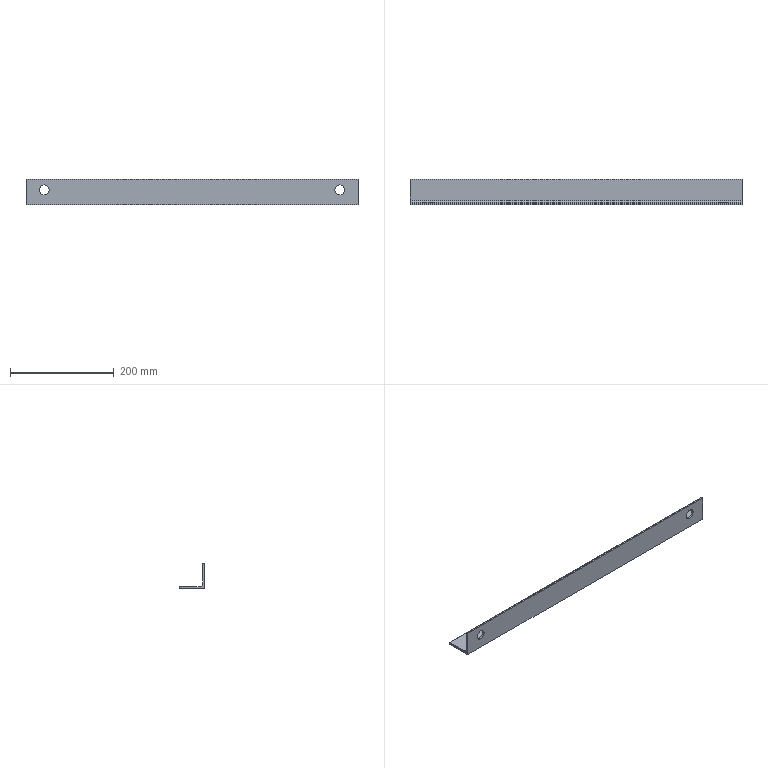Part | STEP file | 粉仓楼梯通道角钢_Default<As Machined> | 1 solid | 15 faces | box 640 x 50 x 50 mm | volume 247161 mm3 | plane 8 | cylinder 7 | commonest cylinder face diameters 19 x4 2.66 x2 11 x1
STEP:
#1=CARTESIAN_POINT('',(0.,0.,0.));
#2=DIRECTION('',(0.,0.,1.));
#3=DIRECTION('',(1.,0.,0.));
#4=AXIS2_PLACEMENT_3D('',#1,#2,#3);
#5=CARTESIAN_POINT('',(-285.,0.,38.585));
#6=VERTEX_POINT('',#5);
#7=CARTESIAN_POINT('',(-285.,4.,38.585));
#8=VERTEX_POINT('',#7);
#9=CARTESIAN_POINT('',(-285.,-6.,38.585));
#10=DIRECTION('',(0.,1.,0.));
#11=VECTOR('',#10,1.);
#12=LINE('',#9,#11);
#13=CARTESIAN_POINT('',(-285.,-6.,29.085));
#14=DIRECTION('',(0.,1.,0.));
#15=DIRECTION('',(0.,0.,1.));
#16=AXIS2_PLACEMENT_3D('',#13,#14,#15);
#17=CYLINDRICAL_SURFACE('',#16,9.5);
#18=CARTESIAN_POINT('',(6.283,0.));
#19=DIRECTION('',(0.,1.));
#20=VECTOR('',#19,1.);
#21=LINE('',#18,#20);
#22=(GEOMETRIC_REPRESENTATION_CONTEXT(2)PARAMETRIC_REPRESENTATION_CONTEXT()REPRESENTATION_CONTEXT('',''));
#23=DEFINITIONAL_REPRESENTATION('',(#21),#22);
#24=PCURVE('',#17,#23);
#25=CARTESIAN_POINT('',(-285.,-6.,29.085));
#26=DIRECTION('',(0.,1.,0.));
#27=DIRECTION('',(0.,0.,1.));
#28=AXIS2_PLACEMENT_3D('',#25,#26,#27);
#29=CYLINDRICAL_SURFACE('',#28,9.5);
#30=CARTESIAN_POINT('',(0.,0.));
#31=DIRECTION('',(0.,1.));
#32=VECTOR('',#31,1.);
#33=LINE('',#30,#32);
#34=(GEOMETRIC_REPRESENTATION_CONTEXT(2)PARAMETRIC_REPRESENTATION_CONTEXT()REPRESENTATION_CONTEXT('',''));
#35=DEFINITIONAL_REPRESENTATION('',(#33),#34);
#36=PCURVE('',#29,#35);
#37=SURFACE_CURVE('',#12,(#24,#36),.PCURVE_S1.);
#38=EDGE_CURVE('',#6,#8,#37,.T.);
#39=ORIENTED_EDGE('',*,*,#38,.T.);
#40=CARTESIAN_POINT('',(-285.,4.,19.585));
#41=VERTEX_POINT('',#40);
#42=CARTESIAN_POINT('',(-285.,4.,29.085));
#43=DIRECTION('',(0.,1.,0.));
#44=DIRECTION('',(0.,0.,1.));
#45=AXIS2_PLACEMENT_3D('',#42,#43,#44);
#46=CIRCLE('',#45,9.5);
#47=CARTESIAN_POINT('',(0.,10.));
#48=DIRECTION('',(1.,0.));
#49=VECTOR('',#48,1.);
#50=LINE('',#47,#49);
#51=(GEOMETRIC_REPRESENTATION_CONTEXT(2)PARAMETRIC_REPRESENTATION_CONTEXT()REPRESENTATION_CONTEXT('',''));
#52=DEFINITIONAL_REPRESENTATION('',(#50),#51);
#53=PCURVE('',#17,#52);
#54=CARTESIAN_POINT('',(320.,4.,48.67));
#55=DIRECTION('',(0.,-1.,0.));
#56=DIRECTION('',(1.,0.,0.));
#57=AXIS2_PLACEMENT_3D('',#54,#55,#56);
#58=PLANE('',#57);
#59=CARTESIAN_POINT('',(-605.,-10.085));
#60=CARTESIAN_POINT('',(-588.546,-10.085));
#61=CARTESIAN_POINT('',(-596.773,-24.335));
#62=CARTESIAN_POINT('',(-605.,-38.585));
#63=CARTESIAN_POINT('',(-613.227,-24.335));
#64=CARTESIAN_POINT('',(-621.454,-10.085));
#65=CARTESIAN_POINT('',(-605.,-10.085));
#66=(BOUNDED_CURVE()B_SPLINE_CURVE(2,(#59,#60,#61,#62,#63,#64,#65),.UNSPECIFIED.,.T.,.F.)B_SPLINE_CURVE_WITH_KNOTS((1,2,2,2,2,1),(-2.094,0.,2.094,4.189,6.283,8.378),.UNSPECIFIED.)CURVE()GEOMETRIC_REPRESENTATION_ITEM()RATIONAL_B_SPLINE_CURVE((1.,0.5,1.,0.5,1.,0.5,1.))REPRESENTATION_ITEM(''));
#67=(GEOMETRIC_REPRESENTATION_CONTEXT(2)PARAMETRIC_REPRESENTATION_CONTEXT()REPRESENTATION_CONTEXT('',''));
#68=DEFINITIONAL_REPRESENTATION('',(#66),#67);
#69=PCURVE('',#58,#68);
#70=SURFACE_CURVE('',#46,(#53,#69),.PCURVE_S1.);
#71=EDGE_CURVE('',#41,#8,#70,.T.);
#72=ORIENTED_EDGE('',*,*,#71,.F.);
#73=CARTESIAN_POINT('',(-285.,0.,19.585));
#74=VERTEX_POINT('',#73);
#75=CARTESIAN_POINT('',(-285.,-6.,19.585));
#76=DIRECTION('',(0.,1.,0.));
#77=VECTOR('',#76,1.);
#78=LINE('',#75,#77);
#79=CARTESIAN_POINT('',(3.142,0.));
#80=DIRECTION('',(0.,1.));
#81=VECTOR('',#80,1.);
#82=LINE('',#79,#81);
#83=(GEOMETRIC_REPRESENTATION_CONTEXT(2)PARAMETRIC_REPRESENTATION_CONTEXT()REPRESENTATION_CONTEXT('',''));
#84=DEFINITIONAL_REPRESENTATION('',(#82),#83);
#85=PCURVE('',#17,#84);
#86=CARTESIAN_POINT('',(3.142,0.));
#87=DIRECTION('',(0.,1.));
#88=VECTOR('',#87,1.);
#89=LINE('',#86,#88);
#90=(GEOMETRIC_REPRESENTATION_CONTEXT(2)PARAMETRIC_REPRESENTATION_CONTEXT()REPRESENTATION_CONTEXT('',''));
#91=DEFINITIONAL_REPRESENTATION('',(#89),#90);
#92=PCURVE('',#29,#91);
#93=SURFACE_CURVE('',#78,(#85,#92),.PCURVE_S1.);
#94=EDGE_CURVE('',#74,#41,#93,.T.);
#95=ORIENTED_EDGE('',*,*,#94,.F.);
#96=CARTESIAN_POINT('',(-285.,0.,29.085));
#97=DIRECTION('',(0.,1.,0.));
#98=DIRECTION('',(-1.,0.,0.));
#99=AXIS2_PLACEMENT_3D('',#96,#97,#98);
#100=CIRCLE('',#99,9.5);
#101=CARTESIAN_POINT('',(-1.571,6.));
#102=DIRECTION('',(1.,0.));
#103=VECTOR('',#102,1.);
#104=LINE('',#101,#103);
#105=(GEOMETRIC_REPRESENTATION_CONTEXT(2)PARAMETRIC_REPRESENTATION_CONTEXT()REPRESENTATION_CONTEXT('',''));
#106=DEFINITIONAL_REPRESENTATION('',(#104),#105);
#107=PCURVE('',#17,#106);
#108=CARTESIAN_POINT('',(320.,0.,50.));
#109=DIRECTION('',(0.,1.,0.));
#110=DIRECTION('',(-1.,0.,0.));
#111=AXIS2_PLACEMENT_3D('',#108,#109,#110);
#112=PLANE('',#111);
#113=CARTESIAN_POINT('',(605.,-20.915));
#114=DIRECTION('',(1.,0.));
#115=AXIS2_PLACEMENT_2D('',#113,#114);
#116=CIRCLE('',#115,9.5);
#117=(GEOMETRIC_REPRESENTATION_CONTEXT(2)PARAMETRIC_REPRESENTATION_CONTEXT()REPRESENTATION_CONTEXT('',''));
#118=DEFINITIONAL_REPRESENTATION('',(#116),#117);
#119=PCURVE('',#112,#118);
#120=SURFACE_CURVE('',#100,(#107,#119),.PCURVE_S1.);
#121=EDGE_CURVE('',#74,#6,#120,.T.);
#122=ORIENTED_EDGE('',*,*,#121,.T.);
#123=EDGE_LOOP('',(#39,#72,#95,#122));
#124=FACE_BOUND('',#123,.F.);
#125=ADVANCED_FACE('',(#124),#17,.F.);
#126=CARTESIAN_POINT('',(285.,0.,38.585));
#127=VERTEX_POINT('',#126);
#128=CARTESIAN_POINT('',(285.,4.,38.585));
#129=VERTEX_POINT('',#128);
#130=CARTESIAN_POINT('',(285.,-6.,38.585));
#131=DIRECTION('',(0.,1.,0.));
#132=VECTOR('',#131,1.);
#133=LINE('',#130,#132);
#134=CARTESIAN_POINT('',(285.,-6.,29.085));
#135=DIRECTION('',(0.,1.,0.));
#136=DIRECTION('',(0.,0.,1.));
#137=AXIS2_PLACEMENT_3D('',#134,#135,#136);
#138=CYLINDRICAL_SURFACE('',#137,9.5);
#139=CARTESIAN_POINT('',(6.283,0.));
#140=DIRECTION('',(0.,1.));
#141=VECTOR('',#140,1.);
#142=LINE('',#139,#141);
#143=(GEOMETRIC_REPRESENTATION_CONTEXT(2)PARAMETRIC_REPRESENTATION_CONTEXT()REPRESENTATION_CONTEXT('',''));
#144=DEFINITIONAL_REPRESENTATION('',(#142),#143);
#145=PCURVE('',#138,#144);
#146=CARTESIAN_POINT('',(285.,-6.,29.085));
#147=DIRECTION('',(0.,1.,0.));
#148=DIRECTION('',(0.,0.,1.));
#149=AXIS2_PLACEMENT_3D('',#146,#147,#148);
#150=CYLINDRICAL_SURFACE('',#149,9.5);
#151=CARTESIAN_POINT('',(0.,0.));
#152=DIRECTION('',(0.,1.));
#153=VECTOR('',#152,1.);
#154=LINE('',#151,#153);
#155=(GEOMETRIC_REPRESENTATION_CONTEXT(2)PARAMETRIC_REPRESENTATION_CONTEXT()REPRESENTATION_CONTEXT('',''));
#156=DEFINITIONAL_REPRESENTATION('',(#154),#155);
#157=PCURVE('',#150,#156);
#158=SURFACE_CURVE('',#133,(#145,#157),.PCURVE_S1.);
#159=EDGE_CURVE('',#127,#129,#158,.T.);
#160=ORIENTED_EDGE('',*,*,#159,.T.);
#161=CARTESIAN_POINT('',(285.,4.,19.585));
#162=VERTEX_POINT('',#161);
#163=CARTESIAN_POINT('',(285.,4.,29.085));
#164=DIRECTION('',(0.,1.,0.));
#165=DIRECTION('',(0.,0.,-1.));
#166=AXIS2_PLACEMENT_3D('',#163,#164,#165);
#167=CIRCLE('',#166,9.5);
#168=CARTESIAN_POINT('',(3.142,10.));
#169=DIRECTION('',(1.,0.));
#170=VECTOR('',#169,1.);
#171=LINE('',#168,#170);
#172=(GEOMETRIC_REPRESENTATION_CONTEXT(2)PARAMETRIC_REPRESENTATION_CONTEXT()REPRESENTATION_CONTEXT('',''));
#173=DEFINITIONAL_REPRESENTATION('',(#171),#172);
#174=PCURVE('',#138,#173);
#175=CARTESIAN_POINT('',(-35.,-29.085));
#176=CARTESIAN_POINT('',(-51.454,-29.085));
#177=CARTESIAN_POINT('',(-43.227,-14.835));
#178=CARTESIAN_POINT('',(-35.,-0.585));
#179=CARTESIAN_POINT('',(-26.773,-14.835));
#180=CARTESIAN_POINT('',(-18.546,-29.085));
#181=CARTESIAN_POINT('',(-35.,-29.085));
#182=(BOUNDED_CURVE()B_SPLINE_CURVE(2,(#175,#176,#177,#178,#179,#180,#181),.UNSPECIFIED.,.T.,.F.)B_SPLINE_CURVE_WITH_KNOTS((1,2,2,2,2,1),(-2.094,0.,2.094,4.189,6.283,8.378),.UNSPECIFIED.)CURVE()GEOMETRIC_REPRESENTATION_ITEM()RATIONAL_B_SPLINE_CURVE((1.,0.5,1.,0.5,1.,0.5,1.))REPRESENTATION_ITEM(''));
#183=(GEOMETRIC_REPRESENTATION_CONTEXT(2)PARAMETRIC_REPRESENTATION_CONTEXT()REPRESENTATION_CONTEXT('',''));
#184=DEFINITIONAL_REPRESENTATION('',(#182),#183);
#185=PCURVE('',#58,#184);
#186=SURFACE_CURVE('',#167,(#174,#185),.PCURVE_S1.);
#187=EDGE_CURVE('',#162,#129,#186,.T.);
#188=ORIENTED_EDGE('',*,*,#187,.F.);
#189=CARTESIAN_POINT('',(285.,0.,19.585));
#190=VERTEX_POINT('',#189);
#191=CARTESIAN_POINT('',(285.,-6.,19.585));
#192=DIRECTION('',(0.,1.,0.));
#193=VECTOR('',#192,1.);
#194=LINE('',#191,#193);
#195=CARTESIAN_POINT('',(3.142,0.));
#196=DIRECTION('',(0.,1.));
#197=VECTOR('',#196,1.);
#198=LINE('',#195,#197);
#199=(GEOMETRIC_REPRESENTATION_CONTEXT(2)PARAMETRIC_REPRESENTATION_CONTEXT()REPRESENTATION_CONTEXT('',''));
#200=DEFINITIONAL_REPRESENTATION('',(#198),#199);
#201=PCURVE('',#138,#200);
#202=CARTESIAN_POINT('',(3.142,0.));
#203=DIRECTION('',(0.,1.));
#204=VECTOR('',#203,1.);
#205=LINE('',#202,#204);
#206=(GEOMETRIC_REPRESENTATION_CONTEXT(2)PARAMETRIC_REPRESENTATION_CONTEXT()REPRESENTATION_CONTEXT('',''));
#207=DEFINITIONAL_REPRESENTATION('',(#205),#206);
#208=PCURVE('',#150,#207);
#209=SURFACE_CURVE('',#194,(#201,#208),.PCURVE_S1.);
#210=EDGE_CURVE('',#190,#162,#209,.T.);
#211=ORIENTED_EDGE('',*,*,#210,.F.);
#212=CARTESIAN_POINT('',(285.,0.,29.085));
#213=DIRECTION('',(0.,1.,0.));
#214=DIRECTION('',(-1.,0.,0.));
#215=AXIS2_PLACEMENT_3D('',#212,#213,#214);
#216=CIRCLE('',#215,9.5);
#217=CARTESIAN_POINT('',(-1.571,6.));
#218=DIRECTION('',(1.,0.));
#219=VECTOR('',#218,1.);
#220=LINE('',#217,#219);
#221=(GEOMETRIC_REPRESENTATION_CONTEXT(2)PARAMETRIC_REPRESENTATION_CONTEXT()REPRESENTATION_CONTEXT('',''));
#222=DEFINITIONAL_REPRESENTATION('',(#220),#221);
#223=PCURVE('',#138,#222);
#224=CARTESIAN_POINT('',(35.,-20.915));
#225=DIRECTION('',(1.,0.));
#226=AXIS2_PLACEMENT_2D('',#224,#225);
#227=CIRCLE('',#226,9.5);
#228=(GEOMETRIC_REPRESENTATION_CONTEXT(2)PARAMETRIC_REPRESENTATION_CONTEXT()REPRESENTATION_CONTEXT('',''));
#229=DEFINITIONAL_REPRESENTATION('',(#227),#228);
#230=PCURVE('',#112,#229);
#231=SURFACE_CURVE('',#216,(#223,#230),.PCURVE_S1.);
#232=EDGE_CURVE('',#190,#127,#231,.T.);
#233=ORIENTED_EDGE('',*,*,#232,.T.);
#234=EDGE_LOOP('',(#160,#188,#211,#233));
#235=FACE_BOUND('',#234,.F.);
#236=ADVANCED_FACE('',(#235),#138,.F.);
#237=CARTESIAN_POINT('',(-320.,50.,2.67));
#238=VERTEX_POINT('',#237);
#239=CARTESIAN_POINT('',(-320.,48.67,4.));
#240=VERTEX_POINT('',#239);
#241=CARTESIAN_POINT('',(-320.,48.67,2.67));
#242=DIRECTION('',(1.,0.,0.));
#243=DIRECTION('',(0.,1.,0.));
#244=AXIS2_PLACEMENT_3D('',#241,#242,#243);
#245=CIRCLE('',#244,1.33);
#246=CARTESIAN_POINT('',(320.,48.67,2.67));
#247=DIRECTION('',(-1.,0.,0.));
#248=DIRECTION('',(0.,-1.,0.));
#249=AXIS2_PLACEMENT_3D('',#246,#247,#248);
#250=CYLINDRICAL_SURFACE('',#249,1.33);
#251=CARTESIAN_POINT('',(3.142,640.));
#252=DIRECTION('',(-1.,0.));
#253=VECTOR('',#252,1.);
#254=LINE('',#251,#253);
#255=(GEOMETRIC_REPRESENTATION_CONTEXT(2)PARAMETRIC_REPRESENTATION_CONTEXT()REPRESENTATION_CONTEXT('',''));
#256=DEFINITIONAL_REPRESENTATION('',(#254),#255);
#257=PCURVE('',#250,#256);
#258=CARTESIAN_POINT('',(-320.,48.67,2.67));
#259=DIRECTION('',(1.,0.,0.));
#260=DIRECTION('',(0.,1.,0.));
#261=AXIS2_PLACEMENT_3D('',#258,#259,#260);
#262=PLANE('',#261);
#263=CARTESIAN_POINT('',(0.,0.));
#264=DIRECTION('',(1.,0.));
#265=AXIS2_PLACEMENT_2D('',#263,#264);
#266=CIRCLE('',#265,1.33);
#267=(GEOMETRIC_REPRESENTATION_CONTEXT(2)PARAMETRIC_REPRESENTATION_CONTEXT()REPRESENTATION_CONTEXT('',''));
#268=DEFINITIONAL_REPRESENTATION('',(#266),#267);
#269=PCURVE('',#262,#268);
#270=SURFACE_CURVE('',#245,(#257,#269),.PCURVE_S1.);
#271=EDGE_CURVE('',#238,#240,#270,.T.);
#272=ORIENTED_EDGE('',*,*,#271,.T.);
#273=CARTESIAN_POINT('',(320.,48.67,4.));
#274=VERTEX_POINT('',#273);
#275=CARTESIAN_POINT('',(320.,48.67,4.));
#276=DIRECTION('',(-1.,0.,0.));
#277=VECTOR('',#276,1.);
#278=LINE('',#275,#277);
#279=CARTESIAN_POINT('',(1.571,0.));
#280=DIRECTION('',(0.,1.));
#281=VECTOR('',#280,1.);
#282=LINE('',#279,#281);
#283=(GEOMETRIC_REPRESENTATION_CONTEXT(2)PARAMETRIC_REPRESENTATION_CONTEXT()REPRESENTATION_CONTEXT('',''));
#284=DEFINITIONAL_REPRESENTATION('',(#282),#283);
#285=PCURVE('',#250,#284);
#286=CARTESIAN_POINT('',(320.,9.5,4.));
#287=DIRECTION('',(0.,0.,-1.));
#288=DIRECTION('',(-1.,0.,0.));
#289=AXIS2_PLACEMENT_3D('',#286,#287,#288);
#290=PLANE('',#289);
#291=CARTESIAN_POINT('',(0.,39.17));
#292=DIRECTION('',(1.,0.));
#293=VECTOR('',#292,1.);
#294=LINE('',#291,#293);
#295=(GEOMETRIC_REPRESENTATION_CONTEXT(2)PARAMETRIC_REPRESENTATION_CONTEXT()REPRESENTATION_CONTEXT('',''));
#296=DEFINITIONAL_REPRESENTATION('',(#294),#295);
#297=PCURVE('',#290,#296);
#298=SURFACE_CURVE('',#278,(#285,#297),.PCURVE_S1.);
#299=EDGE_CURVE('',#274,#240,#298,.T.);
#300=ORIENTED_EDGE('',*,*,#299,.F.);
#301=CARTESIAN_POINT('',(320.,50.,2.67));
#302=VERTEX_POINT('',#301);
#303=CARTESIAN_POINT('',(320.,48.67,2.67));
#304=DIRECTION('',(1.,0.,0.));
#305=DIRECTION('',(0.,1.,0.));
#306=AXIS2_PLACEMENT_3D('',#303,#304,#305);
#307=CIRCLE('',#306,1.33);
#308=CARTESIAN_POINT('',(3.142,0.));
#309=DIRECTION('',(-1.,0.));
#310=VECTOR('',#309,1.);
#311=LINE('',#308,#310);
#312=(GEOMETRIC_REPRESENTATION_CONTEXT(2)PARAMETRIC_REPRESENTATION_CONTEXT()REPRESENTATION_CONTEXT('',''));
#313=DEFINITIONAL_REPRESENTATION('',(#311),#312);
#314=PCURVE('',#250,#313);
#315=CARTESIAN_POINT('',(320.,48.67,2.67));
#316=DIRECTION('',(1.,0.,0.));
#317=DIRECTION('',(0.,1.,0.));
#318=AXIS2_PLACEMENT_3D('',#315,#316,#317);
#319=PLANE('',#318);
#320=CARTESIAN_POINT('',(0.,0.));
#321=DIRECTION('',(1.,0.));
#322=AXIS2_PLACEMENT_2D('',#320,#321);
#323=CIRCLE('',#322,1.33);
#324=(GEOMETRIC_REPRESENTATION_CONTEXT(2)PARAMETRIC_REPRESENTATION_CONTEXT()REPRESENTATION_CONTEXT('',''));
#325=DEFINITIONAL_REPRESENTATION('',(#323),#324);
#326=PCURVE('',#319,#325);
#327=SURFACE_CURVE('',#307,(#314,#326),.PCURVE_S1.);
#328=EDGE_CURVE('',#302,#274,#327,.T.);
#329=ORIENTED_EDGE('',*,*,#328,.F.);
#330=CARTESIAN_POINT('',(320.,50.,2.67));
#331=DIRECTION('',(-1.,0.,0.));
#332=VECTOR('',#331,1.);
#333=LINE('',#330,#332);
#334=CARTESIAN_POINT('',(3.142,0.));
#335=DIRECTION('',(0.,1.));
#336=VECTOR('',#335,1.);
#337=LINE('',#334,#336);
#338=(GEOMETRIC_REPRESENTATION_CONTEXT(2)PARAMETRIC_REPRESENTATION_CONTEXT()REPRESENTATION_CONTEXT('',''));
#339=DEFINITIONAL_REPRESENTATION('',(#337),#338);
#340=PCURVE('',#250,#339);
#341=CARTESIAN_POINT('',(320.,50.,2.67));
#342=DIRECTION('',(0.,-1.,0.));
#343=DIRECTION('',(1.,0.,0.));
#344=AXIS2_PLACEMENT_3D('',#341,#342,#343);
#345=PLANE('',#344);
#346=CARTESIAN_POINT('',(0.,0.));
#347=DIRECTION('',(-1.,0.));
#348=VECTOR('',#347,1.);
#349=LINE('',#346,#348);
#350=(GEOMETRIC_REPRESENTATION_CONTEXT(2)PARAMETRIC_REPRESENTATION_CONTEXT()REPRESENTATION_CONTEXT('',''));
#351=DEFINITIONAL_REPRESENTATION('',(#349),#350);
#352=PCURVE('',#345,#351);
#353=SURFACE_CURVE('',#333,(#340,#352),.PCURVE_S1.);
#354=EDGE_CURVE('',#302,#238,#353,.T.);
#355=ORIENTED_EDGE('',*,*,#354,.T.);
#356=EDGE_LOOP('',(#272,#300,#329,#355));
#357=FACE_BOUND('',#356,.T.);
#358=ADVANCED_FACE('',(#357),#250,.T.);
#359=CARTESIAN_POINT('',(-320.,9.5,4.));
#360=VERTEX_POINT('',#359);
#361=CARTESIAN_POINT('',(-320.,9.5,4.));
#362=DIRECTION('',(0.,-1.,0.));
#363=VECTOR('',#362,1.);
#364=LINE('',#361,#363);
#365=CARTESIAN_POINT('',(640.,0.));
#366=DIRECTION('',(0.,-1.));
#367=VECTOR('',#366,1.);
#368=LINE('',#365,#367);
#369=(GEOMETRIC_REPRESENTATION_CONTEXT(2)PARAMETRIC_REPRESENTATION_CONTEXT()REPRESENTATION_CONTEXT('',''));
#370=DEFINITIONAL_REPRESENTATION('',(#368),#369);
#371=PCURVE('',#290,#370);
#372=CARTESIAN_POINT('',(-39.17,1.33));
#373=DIRECTION('',(-1.,0.));
#374=VECTOR('',#373,1.);
#375=LINE('',#372,#374);
#376=(GEOMETRIC_REPRESENTATION_CONTEXT(2)PARAMETRIC_REPRESENTATION_CONTEXT()REPRESENTATION_CONTEXT('',''));
#377=DEFINITIONAL_REPRESENTATION('',(#375),#376);
#378=PCURVE('',#262,#377);
#379=SURFACE_CURVE('',#364,(#371,#378),.PCURVE_S1.);
#380=EDGE_CURVE('',#240,#360,#379,.T.);
#381=ORIENTED_EDGE('',*,*,#380,.T.);
#382=CARTESIAN_POINT('',(320.,9.5,4.));
#383=VERTEX_POINT('',#382);
#384=CARTESIAN_POINT('',(320.,9.5,4.));
#385=DIRECTION('',(-1.,0.,0.));
#386=VECTOR('',#385,1.);
#387=LINE('',#384,#386);
#388=CARTESIAN_POINT('',(0.,0.));
#389=DIRECTION('',(1.,0.));
#390=VECTOR('',#389,1.);
#391=LINE('',#388,#390);
#392=(GEOMETRIC_REPRESENTATION_CONTEXT(2)PARAMETRIC_REPRESENTATION_CONTEXT()REPRESENTATION_CONTEXT('',''));
#393=DEFINITIONAL_REPRESENTATION('',(#391),#392);
#394=PCURVE('',#290,#393);
#395=CARTESIAN_POINT('',(320.,9.5,9.5));
#396=DIRECTION('',(-1.,0.,0.));
#397=DIRECTION('',(0.,-1.,0.));
#398=AXIS2_PLACEMENT_3D('',#395,#396,#397);
#399=CYLINDRICAL_SURFACE('',#398,5.5);
#400=CARTESIAN_POINT('',(4.712,0.));
#401=DIRECTION('',(0.,1.));
#402=VECTOR('',#401,1.);
#403=LINE('',#400,#402);
#404=(GEOMETRIC_REPRESENTATION_CONTEXT(2)PARAMETRIC_REPRESENTATION_CONTEXT()REPRESENTATION_CONTEXT('',''));
#405=DEFINITIONAL_REPRESENTATION('',(#403),#404);
#406=PCURVE('',#399,#405);
#407=SURFACE_CURVE('',#387,(#394,#406),.PCURVE_S1.);
#408=EDGE_CURVE('',#383,#360,#407,.T.);
#409=ORIENTED_EDGE('',*,*,#408,.F.);
#410=CARTESIAN_POINT('',(320.,9.5,4.));
#411=DIRECTION('',(0.,-1.,0.));
#412=VECTOR('',#411,1.);
#413=LINE('',#410,#412);
#414=CARTESIAN_POINT('',(0.,0.));
#415=DIRECTION('',(0.,-1.));
#416=VECTOR('',#415,1.);
#417=LINE('',#414,#416);
#418=(GEOMETRIC_REPRESENTATION_CONTEXT(2)PARAMETRIC_REPRESENTATION_CONTEXT()REPRESENTATION_CONTEXT('',''));
#419=DEFINITIONAL_REPRESENTATION('',(#417),#418);
#420=PCURVE('',#290,#419);
#421=CARTESIAN_POINT('',(-39.17,1.33));
#422=DIRECTION('',(-1.,0.));
#423=VECTOR('',#422,1.);
#424=LINE('',#421,#423);
#425=(GEOMETRIC_REPRESENTATION_CONTEXT(2)PARAMETRIC_REPRESENTATION_CONTEXT()REPRESENTATION_CONTEXT('',''));
#426=DEFINITIONAL_REPRESENTATION('',(#424),#425);
#427=PCURVE('',#319,#426);
#428=SURFACE_CURVE('',#413,(#420,#427),.PCURVE_S1.);
#429=EDGE_CURVE('',#274,#383,#428,.T.);
#430=ORIENTED_EDGE('',*,*,#429,.F.);
#431=ORIENTED_EDGE('',*,*,#299,.T.);
#432=EDGE_LOOP('',(#381,#409,#430,#431));
#433=FACE_BOUND('',#432,.T.);
#434=ADVANCED_FACE('',(#433),#290,.F.);
#435=ORIENTED_EDGE('',*,*,#408,.F.);
#436=CARTESIAN_POINT('',(320.,4.,9.5));
#437=VERTEX_POINT('',#436);
#438=CARTESIAN_POINT('',(320.,9.5,9.5));
#439=DIRECTION('',(-1.,0.,0.));
#440=DIRECTION('',(0.,1.,0.));
#441=AXIS2_PLACEMENT_3D('',#438,#439,#440);
#442=CIRCLE('',#441,5.5);
#443=CARTESIAN_POINT('',(3.142,0.));
#444=DIRECTION('',(1.,0.));
#445=VECTOR('',#444,1.);
#446=LINE('',#443,#445);
#447=(GEOMETRIC_REPRESENTATION_CONTEXT(2)PARAMETRIC_REPRESENTATION_CONTEXT()REPRESENTATION_CONTEXT('',''));
#448=DEFINITIONAL_REPRESENTATION('',(#446),#447);
#449=PCURVE('',#399,#448);
#450=CARTESIAN_POINT('',(-33.67,6.83));
#451=CARTESIAN_POINT('',(-33.67,-2.696));
#452=CARTESIAN_POINT('',(-41.92,2.067));
#453=CARTESIAN_POINT('',(-50.17,6.83));
#454=CARTESIAN_POINT('',(-41.92,11.593));
#455=CARTESIAN_POINT('',(-33.67,16.356));
#456=CARTESIAN_POINT('',(-33.67,6.83));
#457=(BOUNDED_CURVE()B_SPLINE_CURVE(2,(#450,#451,#452,#453,#454,#455,#456),.UNSPECIFIED.,.T.,.F.)B_SPLINE_CURVE_WITH_KNOTS((1,2,2,2,2,1),(-2.094,0.,2.094,4.189,6.283,8.378),.UNSPECIFIED.)CURVE()GEOMETRIC_REPRESENTATION_ITEM()RATIONAL_B_SPLINE_CURVE((1.,0.5,1.,0.5,1.,0.5,1.))REPRESENTATION_ITEM(''));
#458=(GEOMETRIC_REPRESENTATION_CONTEXT(2)PARAMETRIC_REPRESENTATION_CONTEXT()REPRESENTATION_CONTEXT('',''));
#459=DEFINITIONAL_REPRESENTATION('',(#457),#458);
#460=PCURVE('',#319,#459);
#461=SURFACE_CURVE('',#442,(#449,#460),.PCURVE_S1.);
#462=EDGE_CURVE('',#383,#437,#461,.T.);
#463=ORIENTED_EDGE('',*,*,#462,.T.);
#464=CARTESIAN_POINT('',(-320.,4.,9.5));
#465=VERTEX_POINT('',#464);
#466=CARTESIAN_POINT('',(320.,4.,9.5));
#467=DIRECTION('',(-1.,0.,0.));
#468=VECTOR('',#467,1.);
#469=LINE('',#466,#468);
#470=CARTESIAN_POINT('',(6.283,0.));
#471=DIRECTION('',(0.,1.));
#472=VECTOR('',#471,1.);
#473=LINE('',#470,#472);
#474=(GEOMETRIC_REPRESENTATION_CONTEXT(2)PARAMETRIC_REPRESENTATION_CONTEXT()REPRESENTATION_CONTEXT('',''));
#475=DEFINITIONAL_REPRESENTATION('',(#473),#474);
#476=PCURVE('',#399,#475);
#477=CARTESIAN_POINT('',(0.,-39.17));
#478=DIRECTION('',(-1.,0.));
#479=VECTOR('',#478,1.);
#480=LINE('',#477,#479);
#481=(GEOMETRIC_REPRESENTATION_CONTEXT(2)PARAMETRIC_REPRESENTATION_CONTEXT()REPRESENTATION_CONTEXT('',''));
#482=DEFINITIONAL_REPRESENTATION('',(#480),#481);
#483=PCURVE('',#58,#482);
#484=SURFACE_CURVE('',#469,(#476,#483),.PCURVE_S1.);
#485=EDGE_CURVE('',#437,#465,#484,.T.);
#486=ORIENTED_EDGE('',*,*,#485,.T.);
#487=CARTESIAN_POINT('',(-320.,9.5,9.5));
#488=DIRECTION('',(-1.,0.,0.));
#489=DIRECTION('',(0.,1.,0.));
#490=AXIS2_PLACEMENT_3D('',#487,#488,#489);
#491=CIRCLE('',#490,5.5);
#492=CARTESIAN_POINT('',(3.142,640.));
#493=DIRECTION('',(1.,0.));
#494=VECTOR('',#493,1.);
#495=LINE('',#492,#494);
#496=(GEOMETRIC_REPRESENTATION_CONTEXT(2)PARAMETRIC_REPRESENTATION_CONTEXT()REPRESENTATION_CONTEXT('',''));
#497=DEFINITIONAL_REPRESENTATION('',(#495),#496);
#498=PCURVE('',#399,#497);
#499=CARTESIAN_POINT('',(-33.67,6.83));
#500=CARTESIAN_POINT('',(-33.67,-2.696));
#501=CARTESIAN_POINT('',(-41.92,2.067));
#502=CARTESIAN_POINT('',(-50.17,6.83));
#503=CARTESIAN_POINT('',(-41.92,11.593));
#504=CARTESIAN_POINT('',(-33.67,16.356));
#505=CARTESIAN_POINT('',(-33.67,6.83));
#506=(BOUNDED_CURVE()B_SPLINE_CURVE(2,(#499,#500,#501,#502,#503,#504,#505),.UNSPECIFIED.,.T.,.F.)B_SPLINE_CURVE_WITH_KNOTS((1,2,2,2,2,1),(-2.094,0.,2.094,4.189,6.283,8.378),.UNSPECIFIED.)CURVE()GEOMETRIC_REPRESENTATION_ITEM()RATIONAL_B_SPLINE_CURVE((1.,0.5,1.,0.5,1.,0.5,1.))REPRESENTATION_ITEM(''));
#507=(GEOMETRIC_REPRESENTATION_CONTEXT(2)PARAMETRIC_REPRESENTATION_CONTEXT()REPRESENTATION_CONTEXT('',''));
#508=DEFINITIONAL_REPRESENTATION('',(#506),#507);
#509=PCURVE('',#262,#508);
#510=SURFACE_CURVE('',#491,(#498,#509),.PCURVE_S1.);
#511=EDGE_CURVE('',#360,#465,#510,.T.);
#512=ORIENTED_EDGE('',*,*,#511,.F.);
#513=EDGE_LOOP('',(#435,#463,#486,#512));
#514=FACE_BOUND('',#513,.F.);
#515=ADVANCED_FACE('',(#514),#399,.F.);
#516=CARTESIAN_POINT('',(-285.,4.,29.085));
#517=DIRECTION('',(0.,1.,0.));
#518=DIRECTION('',(0.,0.,1.));
#519=AXIS2_PLACEMENT_3D('',#516,#517,#518);
#520=CIRCLE('',#519,9.5);
#521=CARTESIAN_POINT('',(-605.,-10.085));
#522=CARTESIAN_POINT('',(-588.546,-10.085));
#523=CARTESIAN_POINT('',(-596.773,-24.335));
#524=CARTESIAN_POINT('',(-605.,-38.585));
#525=CARTESIAN_POINT('',(-613.227,-24.335));
#526=CARTESIAN_POINT('',(-621.454,-10.085));
#527=CARTESIAN_POINT('',(-605.,-10.085));
#528=(BOUNDED_CURVE()B_SPLINE_CURVE(2,(#521,#522,#523,#524,#525,#526,#527),.UNSPECIFIED.,.T.,.F.)B_SPLINE_CURVE_WITH_KNOTS((1,2,2,2,2,1),(-2.094,0.,2.094,4.189,6.283,8.378),.UNSPECIFIED.)CURVE()GEOMETRIC_REPRESENTATION_ITEM()RATIONAL_B_SPLINE_CURVE((1.,0.5,1.,0.5,1.,0.5,1.))REPRESENTATION_ITEM(''));
#529=(GEOMETRIC_REPRESENTATION_CONTEXT(2)PARAMETRIC_REPRESENTATION_CONTEXT()REPRESENTATION_CONTEXT('',''));
#530=DEFINITIONAL_REPRESENTATION('',(#528),#529);
#531=PCURVE('',#58,#530);
#532=CARTESIAN_POINT('',(0.,10.));
#533=DIRECTION('',(1.,0.));
#534=VECTOR('',#533,1.);
#535=LINE('',#532,#534);
#536=(GEOMETRIC_REPRESENTATION_CONTEXT(2)PARAMETRIC_REPRESENTATION_CONTEXT()REPRESENTATION_CONTEXT('',''));
#537=DEFINITIONAL_REPRESENTATION('',(#535),#536);
#538=PCURVE('',#29,#537);
#539=SURFACE_CURVE('',#520,(#531,#538),.PCURVE_S1.);
#540=EDGE_CURVE('',#8,#41,#539,.T.);
#541=ORIENTED_EDGE('',*,*,#540,.F.);
#542=ORIENTED_EDGE('',*,*,#71,.F.);
#543=EDGE_LOOP('',(#541,#542));
#544=FACE_BOUND('',#543,.T.);
#545=CARTESIAN_POINT('',(285.,4.,29.085));
#546=DIRECTION('',(0.,1.,0.));
#547=DIRECTION('',(0.,0.,-1.));
#548=AXIS2_PLACEMENT_3D('',#545,#546,#547);
#549=CIRCLE('',#548,9.5);
#550=CARTESIAN_POINT('',(-35.,-29.085));
#551=CARTESIAN_POINT('',(-51.454,-29.085));
#552=CARTESIAN_POINT('',(-43.227,-14.835));
#553=CARTESIAN_POINT('',(-35.,-0.585));
#554=CARTESIAN_POINT('',(-26.773,-14.835));
#555=CARTESIAN_POINT('',(-18.546,-29.085));
#556=CARTESIAN_POINT('',(-35.,-29.085));
#557=(BOUNDED_CURVE()B_SPLINE_CURVE(2,(#550,#551,#552,#553,#554,#555,#556),.UNSPECIFIED.,.T.,.F.)B_SPLINE_CURVE_WITH_KNOTS((1,2,2,2,2,1),(-2.094,0.,2.094,4.189,6.283,8.378),.UNSPECIFIED.)CURVE()GEOMETRIC_REPRESENTATION_ITEM()RATIONAL_B_SPLINE_CURVE((1.,0.5,1.,0.5,1.,0.5,1.))REPRESENTATION_ITEM(''));
#558=(GEOMETRIC_REPRESENTATION_CONTEXT(2)PARAMETRIC_REPRESENTATION_CONTEXT()REPRESENTATION_CONTEXT('',''));
#559=DEFINITIONAL_REPRESENTATION('',(#557),#558);
#560=PCURVE('',#58,#559);
#561=CARTESIAN_POINT('',(-3.142,10.));
#562=DIRECTION('',(1.,0.));
#563=VECTOR('',#562,1.);
#564=LINE('',#561,#563);
#565=(GEOMETRIC_REPRESENTATION_CONTEXT(2)PARAMETRIC_REPRESENTATION_CONTEXT()REPRESENTATION_CONTEXT('',''));
#566=DEFINITIONAL_REPRESENTATION('',(#564),#565);
#567=PCURVE('',#150,#566);
#568=SURFACE_CURVE('',#549,(#560,#567),.PCURVE_S1.);
#569=EDGE_CURVE('',#129,#162,#568,.T.);
#570=ORIENTED_EDGE('',*,*,#569,.F.);
#571=ORIENTED_EDGE('',*,*,#187,.F.);
#572=EDGE_LOOP('',(#570,#571));
#573=FACE_BOUND('',#572,.T.);
#574=CARTESIAN_POINT('',(-320.,4.,48.67));
#575=VERTEX_POINT('',#574);
#576=CARTESIAN_POINT('',(-320.,4.,48.67));
#577=DIRECTION('',(0.,0.,1.));
#578=VECTOR('',#577,1.);
#579=LINE('',#576,#578);
#580=CARTESIAN_POINT('',(-640.,0.));
#581=DIRECTION('',(0.,1.));
#582=VECTOR('',#581,1.);
#583=LINE('',#580,#582);
#584=(GEOMETRIC_REPRESENTATION_CONTEXT(2)PARAMETRIC_REPRESENTATION_CONTEXT()REPRESENTATION_CONTEXT('',''));
#585=DEFINITIONAL_REPRESENTATION('',(#583),#584);
#586=PCURVE('',#58,#585);
#587=CARTESIAN_POINT('',(-44.67,46.));
#588=DIRECTION('',(0.,1.));
#589=VECTOR('',#588,1.);
#590=LINE('',#587,#589);
#591=(GEOMETRIC_REPRESENTATION_CONTEXT(2)PARAMETRIC_REPRESENTATION_CONTEXT()REPRESENTATION_CONTEXT('',''));
#592=DEFINITIONAL_REPRESENTATION('',(#590),#591);
#593=PCURVE('',#262,#592);
#594=SURFACE_CURVE('',#579,(#586,#593),.PCURVE_S1.);
#595=EDGE_CURVE('',#465,#575,#594,.T.);
#596=ORIENTED_EDGE('',*,*,#595,.T.);
#597=CARTESIAN_POINT('',(320.,4.,48.67));
#598=VERTEX_POINT('',#597);
#599=CARTESIAN_POINT('',(320.,4.,48.67));
#600=DIRECTION('',(-1.,0.,0.));
#601=VECTOR('',#600,1.);
#602=LINE('',#599,#601);
#603=CARTESIAN_POINT('',(0.,0.));
#604=DIRECTION('',(-1.,0.));
#605=VECTOR('',#604,1.);
#606=LINE('',#603,#605);
#607=(GEOMETRIC_REPRESENTATION_CONTEXT(2)PARAMETRIC_REPRESENTATION_CONTEXT()REPRESENTATION_CONTEXT('',''));
#608=DEFINITIONAL_REPRESENTATION('',(#606),#607);
#609=PCURVE('',#58,#608);
#610=CARTESIAN_POINT('',(320.,2.67,48.67));
#611=DIRECTION('',(-1.,0.,0.));
#612=DIRECTION('',(0.,-1.,0.));
#613=AXIS2_PLACEMENT_3D('',#610,#611,#612);
#614=CYLINDRICAL_SURFACE('',#613,1.33);
#615=CARTESIAN_POINT('',(3.142,0.));
#616=DIRECTION('',(0.,1.));
#617=VECTOR('',#616,1.);
#618=LINE('',#615,#617);
#619=(GEOMETRIC_REPRESENTATION_CONTEXT(2)PARAMETRIC_REPRESENTATION_CONTEXT()REPRESENTATION_CONTEXT('',''));
#620=DEFINITIONAL_REPRESENTATION('',(#618),#619);
#621=PCURVE('',#614,#620);
#622=SURFACE_CURVE('',#602,(#609,#621),.PCURVE_S1.);
#623=EDGE_CURVE('',#598,#575,#622,.T.);
#624=ORIENTED_EDGE('',*,*,#623,.F.);
#625=CARTESIAN_POINT('',(320.,4.,48.67));
#626=DIRECTION('',(0.,0.,1.));
#627=VECTOR('',#626,1.);
#628=LINE('',#625,#627);
#629=CARTESIAN_POINT('',(0.,0.));
#630=DIRECTION('',(0.,1.));
#631=VECTOR('',#630,1.);
#632=LINE('',#629,#631);
#633=(GEOMETRIC_REPRESENTATION_CONTEXT(2)PARAMETRIC_REPRESENTATION_CONTEXT()REPRESENTATION_CONTEXT('',''));
#634=DEFINITIONAL_REPRESENTATION('',(#632),#633);
#635=PCURVE('',#58,#634);
#636=CARTESIAN_POINT('',(-44.67,46.));
#637=DIRECTION('',(0.,1.));
#638=VECTOR('',#637,1.);
#639=LINE('',#636,#638);
#640=(GEOMETRIC_REPRESENTATION_CONTEXT(2)PARAMETRIC_REPRESENTATION_CONTEXT()REPRESENTATION_CONTEXT('',''));
#641=DEFINITIONAL_REPRESENTATION('',(#639),#640);
#642=PCURVE('',#319,#641);
#643=SURFACE_CURVE('',#628,(#635,#642),.PCURVE_S1.);
#644=EDGE_CURVE('',#437,#598,#643,.T.);
#645=ORIENTED_EDGE('',*,*,#644,.F.);
#646=ORIENTED_EDGE('',*,*,#485,.T.);
#647=EDGE_LOOP('',(#596,#624,#645,#646));
#648=FACE_BOUND('',#647,.T.);
#649=ADVANCED_FACE('',(#544,#573,#648),#58,.F.);
#650=CARTESIAN_POINT('',(-320.,2.67,50.));
#651=VERTEX_POINT('',#650);
#652=CARTESIAN_POINT('',(-320.,2.67,48.67));
#653=DIRECTION('',(1.,0.,0.));
#654=DIRECTION('',(0.,1.,0.));
#655=AXIS2_PLACEMENT_3D('',#652,#653,#654);
#656=CIRCLE('',#655,1.33);
#657=CARTESIAN_POINT('',(3.142,640.));
#658=DIRECTION('',(-1.,0.));
#659=VECTOR('',#658,1.);
#660=LINE('',#657,#659);
#661=(GEOMETRIC_REPRESENTATION_CONTEXT(2)PARAMETRIC_REPRESENTATION_CONTEXT()REPRESENTATION_CONTEXT('',''));
#662=DEFINITIONAL_REPRESENTATION('',(#660),#661);
#663=PCURVE('',#614,#662);
#664=CARTESIAN_POINT('',(-46.,46.));
#665=DIRECTION('',(1.,0.));
#666=AXIS2_PLACEMENT_2D('',#664,#665);
#667=CIRCLE('',#666,1.33);
#668=(GEOMETRIC_REPRESENTATION_CONTEXT(2)PARAMETRIC_REPRESENTATION_CONTEXT()REPRESENTATION_CONTEXT('',''));
#669=DEFINITIONAL_REPRESENTATION('',(#667),#668);
#670=PCURVE('',#262,#669);
#671=SURFACE_CURVE('',#656,(#663,#670),.PCURVE_S1.);
#672=EDGE_CURVE('',#575,#651,#671,.T.);
#673=ORIENTED_EDGE('',*,*,#672,.T.);
#674=CARTESIAN_POINT('',(320.,2.67,50.));
#675=VERTEX_POINT('',#674);
#676=CARTESIAN_POINT('',(320.,2.67,50.));
#677=DIRECTION('',(-1.,0.,0.));
#678=VECTOR('',#677,1.);
#679=LINE('',#676,#678);
#680=CARTESIAN_POINT('',(1.571,0.));
#681=DIRECTION('',(0.,1.));
#682=VECTOR('',#681,1.);
#683=LINE('',#680,#682);
#684=(GEOMETRIC_REPRESENTATION_CONTEXT(2)PARAMETRIC_REPRESENTATION_CONTEXT()REPRESENTATION_CONTEXT('',''));
#685=DEFINITIONAL_REPRESENTATION('',(#683),#684);
#686=PCURVE('',#614,#685);
#687=CARTESIAN_POINT('',(320.,0.,50.));
#688=DIRECTION('',(0.,0.,-1.));
#689=DIRECTION('',(0.,1.,0.));
#690=AXIS2_PLACEMENT_3D('',#687,#688,#689);
#691=PLANE('',#690);
#692=CARTESIAN_POINT('',(2.67,0.));
#693=DIRECTION('',(0.,-1.));
#694=VECTOR('',#693,1.);
#695=LINE('',#692,#694);
#696=(GEOMETRIC_REPRESENTATION_CONTEXT(2)PARAMETRIC_REPRESENTATION_CONTEXT()REPRESENTATION_CONTEXT('',''));
#697=DEFINITIONAL_REPRESENTATION('',(#695),#696);
#698=PCURVE('',#691,#697);
#699=SURFACE_CURVE('',#679,(#686,#698),.PCURVE_S1.);
#700=EDGE_CURVE('',#675,#651,#699,.T.);
#701=ORIENTED_EDGE('',*,*,#700,.F.);
#702=CARTESIAN_POINT('',(320.,2.67,48.67));
#703=DIRECTION('',(1.,0.,0.));
#704=DIRECTION('',(0.,1.,0.));
#705=AXIS2_PLACEMENT_3D('',#702,#703,#704);
#706=CIRCLE('',#705,1.33);
#707=CARTESIAN_POINT('',(3.142,0.));
#708=DIRECTION('',(-1.,0.));
#709=VECTOR('',#708,1.);
#710=LINE('',#707,#709);
#711=(GEOMETRIC_REPRESENTATION_CONTEXT(2)PARAMETRIC_REPRESENTATION_CONTEXT()REPRESENTATION_CONTEXT('',''));
#712=DEFINITIONAL_REPRESENTATION('',(#710),#711);
#713=PCURVE('',#614,#712);
#714=CARTESIAN_POINT('',(-46.,46.));
#715=DIRECTION('',(1.,0.));
#716=AXIS2_PLACEMENT_2D('',#714,#715);
#717=CIRCLE('',#716,1.33);
#718=(GEOMETRIC_REPRESENTATION_CONTEXT(2)PARAMETRIC_REPRESENTATION_CONTEXT()REPRESENTATION_CONTEXT('',''));
#719=DEFINITIONAL_REPRESENTATION('',(#717),#718);
#720=PCURVE('',#319,#719);
#721=SURFACE_CURVE('',#706,(#713,#720),.PCURVE_S1.);
#722=EDGE_CURVE('',#598,#675,#721,.T.);
#723=ORIENTED_EDGE('',*,*,#722,.F.);
#724=ORIENTED_EDGE('',*,*,#623,.T.);
#725=EDGE_LOOP('',(#673,#701,#723,#724));
#726=FACE_BOUND('',#725,.T.);
#727=ADVANCED_FACE('',(#726),#614,.T.);
#728=CARTESIAN_POINT('',(-320.,0.,50.));
#729=VERTEX_POINT('',#728);
#730=CARTESIAN_POINT('',(-320.,0.,50.));
#731=DIRECTION('',(0.,-1.,0.));
#732=VECTOR('',#731,1.);
#733=LINE('',#730,#732);
#734=CARTESIAN_POINT('',(0.,-640.));
#735=DIRECTION('',(-1.,0.));
#736=VECTOR('',#735,1.);
#737=LINE('',#734,#736);
#738=(GEOMETRIC_REPRESENTATION_CONTEXT(2)PARAMETRIC_REPRESENTATION_CONTEXT()REPRESENTATION_CONTEXT('',''));
#739=DEFINITIONAL_REPRESENTATION('',(#737),#738);
#740=PCURVE('',#691,#739);
#741=CARTESIAN_POINT('',(-48.67,47.33));
#742=DIRECTION('',(-1.,0.));
#743=VECTOR('',#742,1.);
#744=LINE('',#741,#743);
#745=(GEOMETRIC_REPRESENTATION_CONTEXT(2)PARAMETRIC_REPRESENTATION_CONTEXT()REPRESENTATION_CONTEXT('',''));
#746=DEFINITIONAL_REPRESENTATION('',(#744),#745);
#747=PCURVE('',#262,#746);
#748=SURFACE_CURVE('',#733,(#740,#747),.PCURVE_S1.);
#749=EDGE_CURVE('',#651,#729,#748,.T.);
#750=ORIENTED_EDGE('',*,*,#749,.T.);
#751=CARTESIAN_POINT('',(320.,0.,50.));
#752=VERTEX_POINT('',#751);
#753=CARTESIAN_POINT('',(320.,0.,50.));
#754=DIRECTION('',(-1.,0.,0.));
#755=VECTOR('',#754,1.);
#756=LINE('',#753,#755);
#757=CARTESIAN_POINT('',(0.,0.));
#758=DIRECTION('',(0.,-1.));
#759=VECTOR('',#758,1.);
#760=LINE('',#757,#759);
#761=(GEOMETRIC_REPRESENTATION_CONTEXT(2)PARAMETRIC_REPRESENTATION_CONTEXT()REPRESENTATION_CONTEXT('',''));
#762=DEFINITIONAL_REPRESENTATION('',(#760),#761);
#763=PCURVE('',#691,#762);
#764=CARTESIAN_POINT('',(0.,0.));
#765=DIRECTION('',(1.,0.));
#766=VECTOR('',#765,1.);
#767=LINE('',#764,#766);
#768=(GEOMETRIC_REPRESENTATION_CONTEXT(2)PARAMETRIC_REPRESENTATION_CONTEXT()REPRESENTATION_CONTEXT('',''));
#769=DEFINITIONAL_REPRESENTATION('',(#767),#768);
#770=PCURVE('',#112,#769);
#771=SURFACE_CURVE('',#756,(#763,#770),.PCURVE_S1.);
#772=EDGE_CURVE('',#752,#729,#771,.T.);
#773=ORIENTED_EDGE('',*,*,#772,.F.);
#774=CARTESIAN_POINT('',(320.,0.,50.));
#775=DIRECTION('',(0.,-1.,0.));
#776=VECTOR('',#775,1.);
#777=LINE('',#774,#776);
#778=CARTESIAN_POINT('',(0.,0.));
#779=DIRECTION('',(-1.,0.));
#780=VECTOR('',#779,1.);
#781=LINE('',#778,#780);
#782=(GEOMETRIC_REPRESENTATION_CONTEXT(2)PARAMETRIC_REPRESENTATION_CONTEXT()REPRESENTATION_CONTEXT('',''));
#783=DEFINITIONAL_REPRESENTATION('',(#781),#782);
#784=PCURVE('',#691,#783);
#785=CARTESIAN_POINT('',(-48.67,47.33));
#786=DIRECTION('',(-1.,0.));
#787=VECTOR('',#786,1.);
#788=LINE('',#785,#787);
#789=(GEOMETRIC_REPRESENTATION_CONTEXT(2)PARAMETRIC_REPRESENTATION_CONTEXT()REPRESENTATION_CONTEXT('',''));
#790=DEFINITIONAL_REPRESENTATION('',(#788),#789);
#791=PCURVE('',#319,#790);
#792=SURFACE_CURVE('',#777,(#784,#791),.PCURVE_S1.);
#793=EDGE_CURVE('',#675,#752,#792,.T.);
#794=ORIENTED_EDGE('',*,*,#793,.F.);
#795=ORIENTED_EDGE('',*,*,#700,.T.);
#796=EDGE_LOOP('',(#750,#773,#794,#795));
#797=FACE_BOUND('',#796,.T.);
#798=ADVANCED_FACE('',(#797),#691,.F.);
#799=CARTESIAN_POINT('',(-285.,0.,29.085));
#800=DIRECTION('',(0.,1.,0.));
#801=DIRECTION('',(-1.,0.,0.));
#802=AXIS2_PLACEMENT_3D('',#799,#800,#801);
#803=CIRCLE('',#802,9.5);
#804=CARTESIAN_POINT('',(605.,-20.915));
#805=DIRECTION('',(1.,0.));
#806=AXIS2_PLACEMENT_2D('',#804,#805);
#807=CIRCLE('',#806,9.5);
#808=(GEOMETRIC_REPRESENTATION_CONTEXT(2)PARAMETRIC_REPRESENTATION_CONTEXT()REPRESENTATION_CONTEXT('',''));
#809=DEFINITIONAL_REPRESENTATION('',(#807),#808);
#810=PCURVE('',#112,#809);
#811=CARTESIAN_POINT('',(-1.571,6.));
#812=DIRECTION('',(1.,0.));
#813=VECTOR('',#812,1.);
#814=LINE('',#811,#813);
#815=(GEOMETRIC_REPRESENTATION_CONTEXT(2)PARAMETRIC_REPRESENTATION_CONTEXT()REPRESENTATION_CONTEXT('',''));
#816=DEFINITIONAL_REPRESENTATION('',(#814),#815);
#817=PCURVE('',#29,#816);
#818=SURFACE_CURVE('',#803,(#810,#817),.PCURVE_S1.);
#819=EDGE_CURVE('',#6,#74,#818,.T.);
#820=ORIENTED_EDGE('',*,*,#819,.T.);
#821=ORIENTED_EDGE('',*,*,#121,.T.);
#822=EDGE_LOOP('',(#820,#821));
#823=FACE_BOUND('',#822,.T.);
#824=CARTESIAN_POINT('',(285.,0.,29.085));
#825=DIRECTION('',(0.,1.,0.));
#826=DIRECTION('',(-1.,0.,0.));
#827=AXIS2_PLACEMENT_3D('',#824,#825,#826);
#828=CIRCLE('',#827,9.5);
#829=CARTESIAN_POINT('',(35.,-20.915));
#830=DIRECTION('',(1.,0.));
#831=AXIS2_PLACEMENT_2D('',#829,#830);
#832=CIRCLE('',#831,9.5);
#833=(GEOMETRIC_REPRESENTATION_CONTEXT(2)PARAMETRIC_REPRESENTATION_CONTEXT()REPRESENTATION_CONTEXT('',''));
#834=DEFINITIONAL_REPRESENTATION('',(#832),#833);
#835=PCURVE('',#112,#834);
#836=CARTESIAN_POINT('',(-1.571,6.));
#837=DIRECTION('',(1.,0.));
#838=VECTOR('',#837,1.);
#839=LINE('',#836,#838);
#840=(GEOMETRIC_REPRESENTATION_CONTEXT(2)PARAMETRIC_REPRESENTATION_CONTEXT()REPRESENTATION_CONTEXT('',''));
#841=DEFINITIONAL_REPRESENTATION('',(#839),#840);
#842=PCURVE('',#150,#841);
#843=SURFACE_CURVE('',#828,(#835,#842),.PCURVE_S1.);
#844=EDGE_CURVE('',#127,#190,#843,.T.);
#845=ORIENTED_EDGE('',*,*,#844,.T.);
#846=ORIENTED_EDGE('',*,*,#232,.T.);
#847=EDGE_LOOP('',(#845,#846));
#848=FACE_BOUND('',#847,.T.);
#849=CARTESIAN_POINT('',(-320.,0.,0.));
#850=VERTEX_POINT('',#849);
#851=CARTESIAN_POINT('',(-320.,0.,50.));
#852=DIRECTION('',(0.,0.,-1.));
#853=VECTOR('',#852,1.);
#854=LINE('',#851,#853);
#855=CARTESIAN_POINT('',(640.,0.));
#856=DIRECTION('',(0.,-1.));
#857=VECTOR('',#856,1.);
#858=LINE('',#855,#857);
#859=(GEOMETRIC_REPRESENTATION_CONTEXT(2)PARAMETRIC_REPRESENTATION_CONTEXT()REPRESENTATION_CONTEXT('',''));
#860=DEFINITIONAL_REPRESENTATION('',(#858),#859);
#861=PCURVE('',#112,#860);
#862=CARTESIAN_POINT('',(-48.67,47.33));
#863=DIRECTION('',(0.,-1.));
#864=VECTOR('',#863,1.);
#865=LINE('',#862,#864);
#866=(GEOMETRIC_REPRESENTATION_CONTEXT(2)PARAMETRIC_REPRESENTATION_CONTEXT()REPRESENTATION_CONTEXT('',''));
#867=DEFINITIONAL_REPRESENTATION('',(#865),#866);
#868=PCURVE('',#262,#867);
#869=SURFACE_CURVE('',#854,(#861,#868),.PCURVE_S1.);
#870=EDGE_CURVE('',#729,#850,#869,.T.);
#871=ORIENTED_EDGE('',*,*,#870,.T.);
#872=CARTESIAN_POINT('',(320.,0.,0.));
#873=VERTEX_POINT('',#872);
#874=CARTESIAN_POINT('',(320.,0.,0.));
#875=DIRECTION('',(-1.,0.,0.));
#876=VECTOR('',#875,1.);
#877=LINE('',#874,#876);
#878=CARTESIAN_POINT('',(0.,-50.));
#879=DIRECTION('',(1.,0.));
#880=VECTOR('',#879,1.);
#881=LINE('',#878,#880);
#882=(GEOMETRIC_REPRESENTATION_CONTEXT(2)PARAMETRIC_REPRESENTATION_CONTEXT()REPRESENTATION_CONTEXT('',''));
#883=DEFINITIONAL_REPRESENTATION('',(#881),#882);
#884=PCURVE('',#112,#883);
#885=CARTESIAN_POINT('',(320.,0.,0.));
#886=DIRECTION('',(0.,0.,1.));
#887=DIRECTION('',(1.,0.,0.));
#888=AXIS2_PLACEMENT_3D('',#885,#886,#887);
#889=PLANE('',#888);
#890=CARTESIAN_POINT('',(0.,0.));
#891=DIRECTION('',(-1.,0.));
#892=VECTOR('',#891,1.);
#893=LINE('',#890,#892);
#894=(GEOMETRIC_REPRESENTATION_CONTEXT(2)PARAMETRIC_REPRESENTATION_CONTEXT()REPRESENTATION_CONTEXT('',''));
#895=DEFINITIONAL_REPRESENTATION('',(#893),#894);
#896=PCURVE('',#889,#895);
#897=SURFACE_CURVE('',#877,(#884,#896),.PCURVE_S1.);
#898=EDGE_CURVE('',#873,#850,#897,.T.);
#899=ORIENTED_EDGE('',*,*,#898,.F.);
#900=CARTESIAN_POINT('',(320.,0.,50.));
#901=DIRECTION('',(0.,0.,-1.));
#902=VECTOR('',#901,1.);
#903=LINE('',#900,#902);
#904=CARTESIAN_POINT('',(0.,0.));
#905=DIRECTION('',(0.,-1.));
#906=VECTOR('',#905,1.);
#907=LINE('',#904,#906);
#908=(GEOMETRIC_REPRESENTATION_CONTEXT(2)PARAMETRIC_REPRESENTATION_CONTEXT()REPRESENTATION_CONTEXT('',''));
#909=DEFINITIONAL_REPRESENTATION('',(#907),#908);
#910=PCURVE('',#112,#909);
#911=CARTESIAN_POINT('',(-48.67,47.33));
#912=DIRECTION('',(0.,-1.));
#913=VECTOR('',#912,1.);
#914=LINE('',#911,#913);
#915=(GEOMETRIC_REPRESENTATION_CONTEXT(2)PARAMETRIC_REPRESENTATION_CONTEXT()REPRESENTATION_CONTEXT('',''));
#916=DEFINITIONAL_REPRESENTATION('',(#914),#915);
#917=PCURVE('',#319,#916);
#918=SURFACE_CURVE('',#903,(#910,#917),.PCURVE_S1.);
#919=EDGE_CURVE('',#752,#873,#918,.T.);
#920=ORIENTED_EDGE('',*,*,#919,.F.);
#921=ORIENTED_EDGE('',*,*,#772,.T.);
#922=EDGE_LOOP('',(#871,#899,#920,#921));
#923=FACE_BOUND('',#922,.T.);
#924=ADVANCED_FACE('',(#823,#848,#923),#112,.F.);
#925=CARTESIAN_POINT('',(-320.,50.,0.));
#926=VERTEX_POINT('',#925);
#927=CARTESIAN_POINT('',(-320.,0.,0.));
#928=DIRECTION('',(0.,1.,0.));
#929=VECTOR('',#928,1.);
#930=LINE('',#927,#929);
#931=CARTESIAN_POINT('',(-640.,0.));
#932=DIRECTION('',(0.,1.));
#933=VECTOR('',#932,1.);
#934=LINE('',#931,#933);
#935=(GEOMETRIC_REPRESENTATION_CONTEXT(2)PARAMETRIC_REPRESENTATION_CONTEXT()REPRESENTATION_CONTEXT('',''));
#936=DEFINITIONAL_REPRESENTATION('',(#934),#935);
#937=PCURVE('',#889,#936);
#938=CARTESIAN_POINT('',(-48.67,-2.67));
#939=DIRECTION('',(1.,0.));
#940=VECTOR('',#939,1.);
#941=LINE('',#938,#940);
#942=(GEOMETRIC_REPRESENTATION_CONTEXT(2)PARAMETRIC_REPRESENTATION_CONTEXT()REPRESENTATION_CONTEXT('',''));
#943=DEFINITIONAL_REPRESENTATION('',(#941),#942);
#944=PCURVE('',#262,#943);
#945=SURFACE_CURVE('',#930,(#937,#944),.PCURVE_S1.);
#946=EDGE_CURVE('',#850,#926,#945,.T.);
#947=ORIENTED_EDGE('',*,*,#946,.T.);
#948=CARTESIAN_POINT('',(320.,50.,0.));
#949=VERTEX_POINT('',#948);
#950=CARTESIAN_POINT('',(320.,50.,0.));
#951=DIRECTION('',(-1.,0.,0.));
#952=VECTOR('',#951,1.);
#953=LINE('',#950,#952);
#954=CARTESIAN_POINT('',(0.,50.));
#955=DIRECTION('',(-1.,0.));
#956=VECTOR('',#955,1.);
#957=LINE('',#954,#956);
#958=(GEOMETRIC_REPRESENTATION_CONTEXT(2)PARAMETRIC_REPRESENTATION_CONTEXT()REPRESENTATION_CONTEXT('',''));
#959=DEFINITIONAL_REPRESENTATION('',(#957),#958);
#960=PCURVE('',#889,#959);
#961=CARTESIAN_POINT('',(0.,-2.67));
#962=DIRECTION('',(-1.,0.));
#963=VECTOR('',#962,1.);
#964=LINE('',#961,#963);
#965=(GEOMETRIC_REPRESENTATION_CONTEXT(2)PARAMETRIC_REPRESENTATION_CONTEXT()REPRESENTATION_CONTEXT('',''));
#966=DEFINITIONAL_REPRESENTATION('',(#964),#965);
#967=PCURVE('',#345,#966);
#968=SURFACE_CURVE('',#953,(#960,#967),.PCURVE_S1.);
#969=EDGE_CURVE('',#949,#926,#968,.T.);
#970=ORIENTED_EDGE('',*,*,#969,.F.);
#971=CARTESIAN_POINT('',(320.,0.,0.));
#972=DIRECTION('',(0.,1.,0.));
#973=VECTOR('',#972,1.);
#974=LINE('',#971,#973);
#975=CARTESIAN_POINT('',(0.,0.));
#976=DIRECTION('',(0.,1.));
#977=VECTOR('',#976,1.);
#978=LINE('',#975,#977);
#979=(GEOMETRIC_REPRESENTATION_CONTEXT(2)PARAMETRIC_REPRESENTATION_CONTEXT()REPRESENTATION_CONTEXT('',''));
#980=DEFINITIONAL_REPRESENTATION('',(#978),#979);
#981=PCURVE('',#889,#980);
#982=CARTESIAN_POINT('',(-48.67,-2.67));
#983=DIRECTION('',(1.,0.));
#984=VECTOR('',#983,1.);
#985=LINE('',#982,#984);
#986=(GEOMETRIC_REPRESENTATION_CONTEXT(2)PARAMETRIC_REPRESENTATION_CONTEXT()REPRESENTATION_CONTEXT('',''));
#987=DEFINITIONAL_REPRESENTATION('',(#985),#986);
#988=PCURVE('',#319,#987);
#989=SURFACE_CURVE('',#974,(#981,#988),.PCURVE_S1.);
#990=EDGE_CURVE('',#873,#949,#989,.T.);
#991=ORIENTED_EDGE('',*,*,#990,.F.);
#992=ORIENTED_EDGE('',*,*,#898,.T.);
#993=EDGE_LOOP('',(#947,#970,#991,#992));
#994=FACE_BOUND('',#993,.T.);
#995=ADVANCED_FACE('',(#994),#889,.F.);
#996=CARTESIAN_POINT('',(-320.,50.,2.67));
#997=DIRECTION('',(0.,0.,1.));
#998=VECTOR('',#997,1.);
#999=LINE('',#996,#998);
#1000=CARTESIAN_POINT('',(-640.,0.));
#1001=DIRECTION('',(0.,1.));
#1002=VECTOR('',#1001,1.);
#1003=LINE('',#1000,#1002);
#1004=(GEOMETRIC_REPRESENTATION_CONTEXT(2)PARAMETRIC_REPRESENTATION_CONTEXT()REPRESENTATION_CONTEXT('',''));
#1005=DEFINITIONAL_REPRESENTATION('',(#1003),#1004);
#1006=PCURVE('',#345,#1005);
#1007=CARTESIAN_POINT('',(1.33,0.));
#1008=DIRECTION('',(0.,1.));
#1009=VECTOR('',#1008,1.);
#1010=LINE('',#1007,#1009);
#1011=(GEOMETRIC_REPRESENTATION_CONTEXT(2)PARAMETRIC_REPRESENTATION_CONTEXT()REPRESENTATION_CONTEXT('',''));
#1012=DEFINITIONAL_REPRESENTATION('',(#1010),#1011);
#1013=PCURVE('',#262,#1012);
#1014=SURFACE_CURVE('',#999,(#1006,#1013),.PCURVE_S1.);
#1015=EDGE_CURVE('',#926,#238,#1014,.T.);
#1016=ORIENTED_EDGE('',*,*,#1015,.T.);
#1017=ORIENTED_EDGE('',*,*,#354,.F.);
#1018=CARTESIAN_POINT('',(320.,50.,2.67));
#1019=DIRECTION('',(0.,0.,1.));
#1020=VECTOR('',#1019,1.);
#1021=LINE('',#1018,#1020);
#1022=CARTESIAN_POINT('',(0.,0.));
#1023=DIRECTION('',(0.,1.));
#1024=VECTOR('',#1023,1.);
#1025=LINE('',#1022,#1024);
#1026=(GEOMETRIC_REPRESENTATION_CONTEXT(2)PARAMETRIC_REPRESENTATION_CONTEXT()REPRESENTATION_CONTEXT('',''));
#1027=DEFINITIONAL_REPRESENTATION('',(#1025),#1026);
#1028=PCURVE('',#345,#1027);
#1029=CARTESIAN_POINT('',(1.33,0.));
#1030=DIRECTION('',(0.,1.));
#1031=VECTOR('',#1030,1.);
#1032=LINE('',#1029,#1031);
#1033=(GEOMETRIC_REPRESENTATION_CONTEXT(2)PARAMETRIC_REPRESENTATION_CONTEXT()REPRESENTATION_CONTEXT('',''));
#1034=DEFINITIONAL_REPRESENTATION('',(#1032),#1033);
#1035=PCURVE('',#319,#1034);
#1036=SURFACE_CURVE('',#1021,(#1028,#1035),.PCURVE_S1.);
#1037=EDGE_CURVE('',#949,#302,#1036,.T.);
#1038=ORIENTED_EDGE('',*,*,#1037,.F.);
#1039=ORIENTED_EDGE('',*,*,#969,.T.);
#1040=EDGE_LOOP('',(#1016,#1017,#1038,#1039));
#1041=FACE_BOUND('',#1040,.T.);
#1042=ADVANCED_FACE('',(#1041),#345,.F.);
#1043=ORIENTED_EDGE('',*,*,#328,.T.);
#1044=ORIENTED_EDGE('',*,*,#429,.T.);
#1045=ORIENTED_EDGE('',*,*,#462,.T.);
#1046=ORIENTED_EDGE('',*,*,#644,.T.);
#1047=ORIENTED_EDGE('',*,*,#722,.T.);
#1048=ORIENTED_EDGE('',*,*,#793,.T.);
#1049=ORIENTED_EDGE('',*,*,#919,.T.);
#1050=ORIENTED_EDGE('',*,*,#990,.T.);
#1051=ORIENTED_EDGE('',*,*,#1037,.T.);
#1052=EDGE_LOOP('',(#1043,#1044,#1045,#1046,#1047,#1048,#1049,#1050,#1051));
#1053=FACE_BOUND('',#1052,.T.);
#1054=ADVANCED_FACE('',(#1053),#319,.T.);
#1055=ORIENTED_EDGE('',*,*,#271,.F.);
#1056=ORIENTED_EDGE('',*,*,#1015,.F.);
#1057=ORIENTED_EDGE('',*,*,#946,.F.);
#1058=ORIENTED_EDGE('',*,*,#870,.F.);
#1059=ORIENTED_EDGE('',*,*,#749,.F.);
#1060=ORIENTED_EDGE('',*,*,#672,.F.);
#1061=ORIENTED_EDGE('',*,*,#595,.F.);
#1062=ORIENTED_EDGE('',*,*,#511,.F.);
#1063=ORIENTED_EDGE('',*,*,#380,.F.);
#1064=EDGE_LOOP('',(#1055,#1056,#1057,#1058,#1059,#1060,#1061,#1062,#1063));
#1065=FACE_BOUND('',#1064,.T.);
#1066=ADVANCED_FACE('',(#1065),#262,.F.);
#1067=ORIENTED_EDGE('',*,*,#569,.F.);
#1068=ORIENTED_EDGE('',*,*,#159,.F.);
#1069=ORIENTED_EDGE('',*,*,#844,.T.);
#1070=ORIENTED_EDGE('',*,*,#210,.T.);
#1071=EDGE_LOOP('',(#1067,#1068,#1069,#1070));
#1072=FACE_BOUND('',#1071,.F.);
#1073=ADVANCED_FACE('',(#1072),#150,.F.);
#1074=ORIENTED_EDGE('',*,*,#540,.F.);
#1075=ORIENTED_EDGE('',*,*,#38,.F.);
#1076=ORIENTED_EDGE('',*,*,#819,.T.);
#1077=ORIENTED_EDGE('',*,*,#94,.T.);
#1078=EDGE_LOOP('',(#1074,#1075,#1076,#1077));
#1079=FACE_BOUND('',#1078,.F.);
#1080=ADVANCED_FACE('',(#1079),#29,.F.);
#1081=CLOSED_SHELL('',(#125,#236,#358,#434,#515,#649,#727,#798,#924,#995,#1042,#1054,#1066,#1073,#1080));
#1082=MANIFOLD_SOLID_BREP('',#1081);
#1083=(LENGTH_UNIT()NAMED_UNIT(*)SI_UNIT(.MILLI.,.METRE.));
#1084=UNCERTAINTY_MEASURE_WITH_UNIT(LENGTH_MEASURE(0.0000001),#1083,'','');
#1085=(NAMED_UNIT(*)PLANE_ANGLE_UNIT()SI_UNIT($,.RADIAN.));
#1086=(NAMED_UNIT(*)SI_UNIT($,.STERADIAN.)SOLID_ANGLE_UNIT());
#1087=(GEOMETRIC_REPRESENTATION_CONTEXT(3)GLOBAL_UNCERTAINTY_ASSIGNED_CONTEXT((#1084))GLOBAL_UNIT_ASSIGNED_CONTEXT((#1083,#1085,#1086))REPRESENTATION_CONTEXT('',''));
#1088=ADVANCED_BREP_SHAPE_REPRESENTATION('',(#4,#1082),#1087);